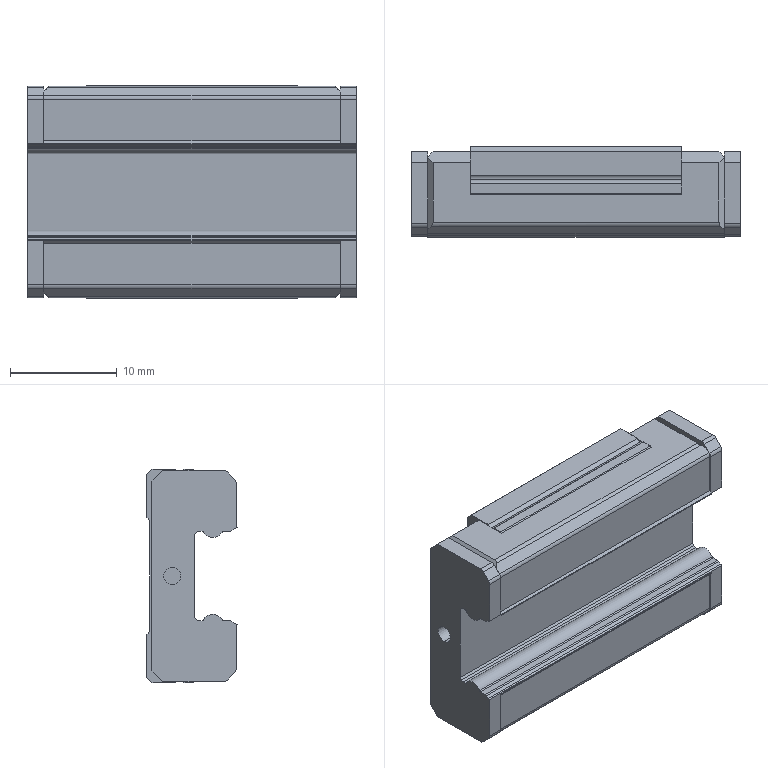Part | SolidWorks | features BaseBody 1 | 1 solid | 146 faces | box 30.8 x 8.5 x 20 mm | volume 3834 mm3 | plane 88 | cylinder 42 | cone 16 | commonest cylinder face diameters 1 x17 2.459 x8 0.6 x6 0.3 x4 1.6 x4 2 x3